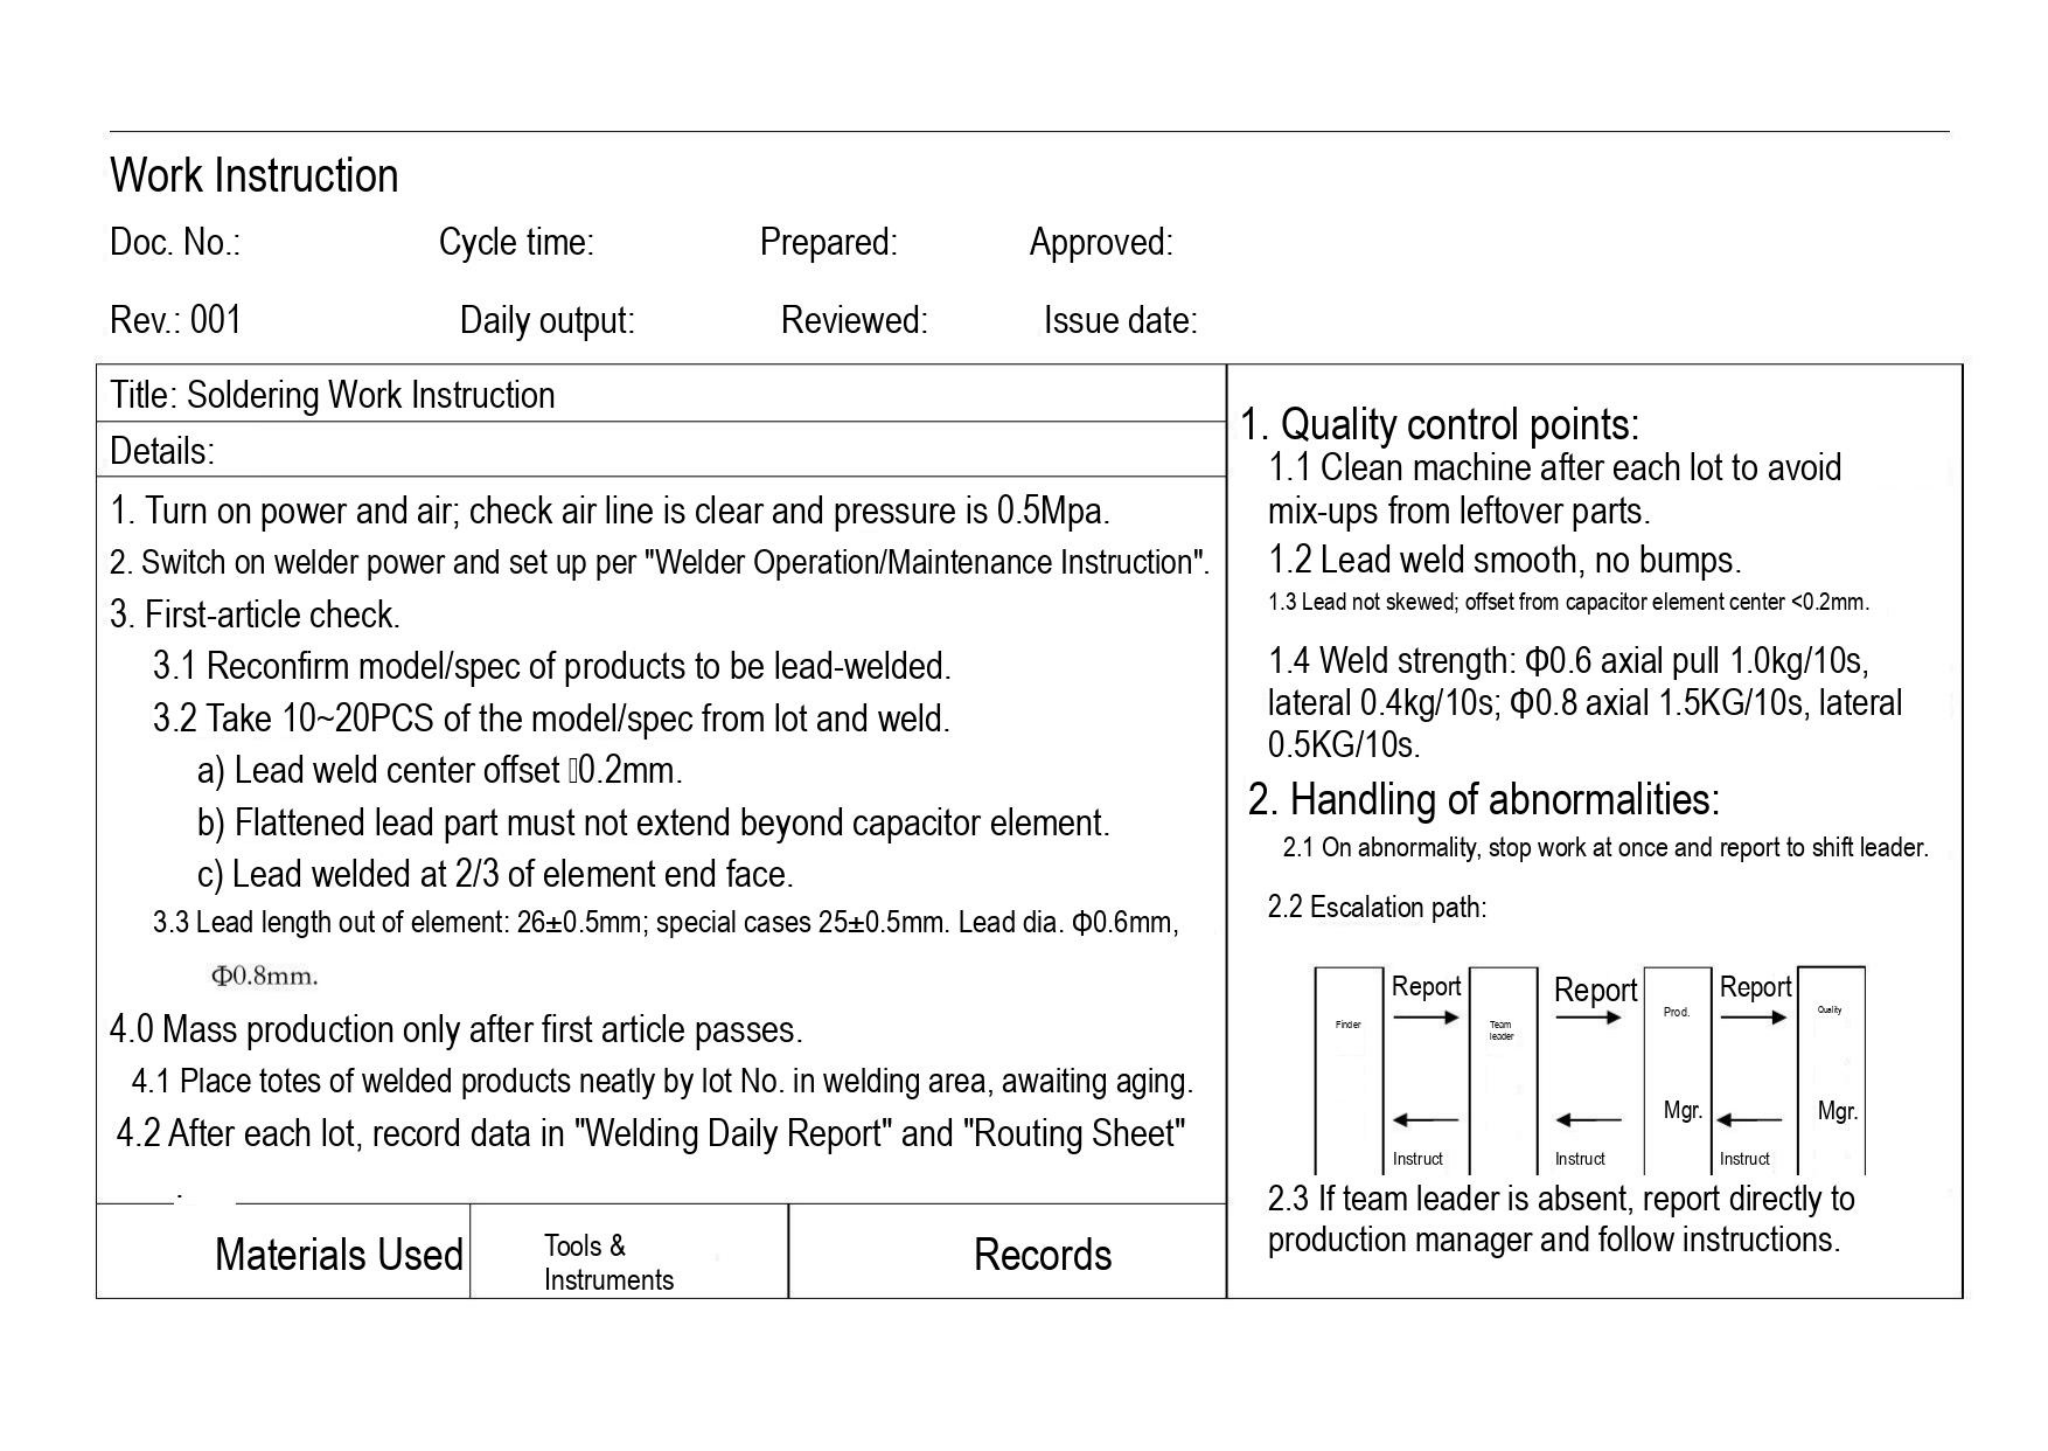Work Instruction

Doc. No.: Cycle time: Prepared: Approved:

Rev.: 001 Daily output: Reviewed: Issue date:

Title: Soldering Work Instruction

Details:

1. Turn on power and air; check air line is clear and pressure is 0.5Mpa.
2. Switch on welder power and set up per "Welder Operation/Maintenance Instruction".
3. First-article check.
 3.1 Reconfirm model/spec of products to be lead-welded.
 3.2 Take 10~20PCS of the model/spec from lot and weld.
  a) Lead weld center offset 0.2mm.
  b) Flattened lead part must not extend beyond capacitor element.
  c) Lead welded at 2/3 of element end face.
 3.3 Lead length out of element: 26±0.5mm; special cases 25±0.5mm. Lead dia. Φ0.6mm, Φ0.8mm.

4.0 Mass production only after first article passes.
 4.1 Place totes of welded products neatly by lot No. in welding area, awaiting aging.
 4.2 After each lot, record data in "Welding Daily Report" and "Routing Sheet"

| Materials Used | Tools & Instruments | Records |
|---|---|---|

1. Quality control points:
 1.1 Clean machine after each lot to avoid mix-ups from leftover parts.
 1.2 Lead weld smooth, no bumps.
 1.3 Lead not skewed; offset from capacitor element center <0.2mm.
 1.4 Weld strength: Φ0.6 axial pull 1.0kg/10s, lateral 0.4kg/10s; Φ0.8 axial 1.5KG/10s, lateral 0.5KG/10s.

2. Handling of abnormalities:
 2.1 On abnormality, stop work at once and report to shift leader.
 2.2 Escalation path:

Finder — Report → Team leader — Report → Prod. Mgr. — Report → Quality Mgr.
Instruct Instruct Instruct

 2.3 If team leader is absent, report directly to production manager and follow instructions.